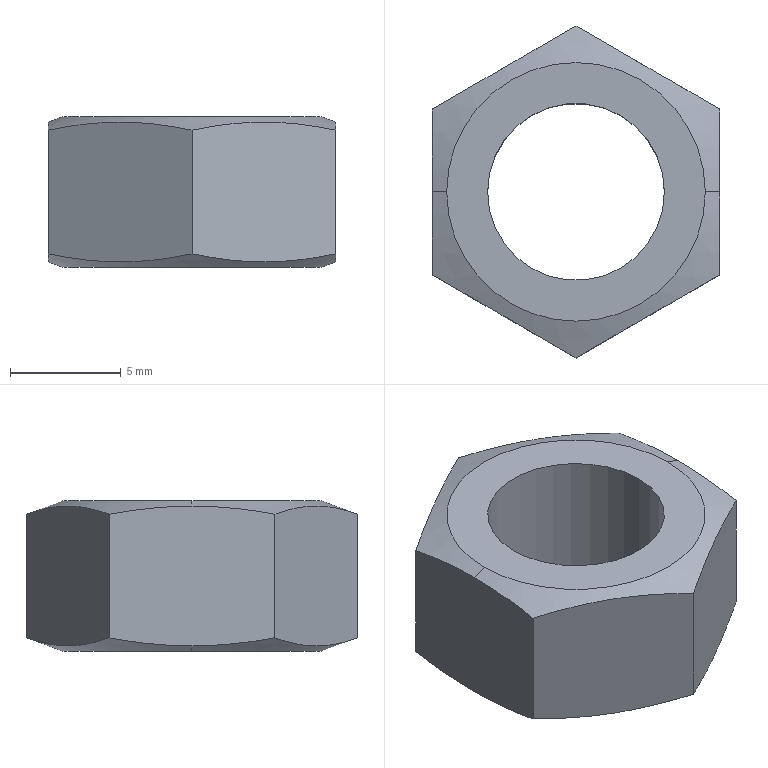Part | SolidWorks | features Extrusion 1, ICE 1, MirrorPattern 1, RefAxis 1, RevCut 1 | 1 solid | 14 faces | box 13 x 15.011 x 6.8 mm | volume 637.901 mm3 | plane 8 | cone 4 | cylinder 2 | commonest cylinder face diameters 8 x2
STEP:
#1=CARTESIAN_POINT('',(-4.,0.,0.));
#2=VERTEX_POINT('',#1);
#3=CARTESIAN_POINT('',(4.,0.,0.));
#4=VERTEX_POINT('',#3);
#5=CARTESIAN_POINT('',(0.,0.,0.));
#6=DIRECTION('',(0.,0.,1.));
#7=DIRECTION('',(1.,0.,0.));
#8=AXIS2_PLACEMENT_3D('',#5,#6,#7);
#9=CIRCLE('',#8,4.);
#10=EDGE_CURVE('',#2,#4,#9,.T.);
#11=ORIENTED_EDGE('',*,*,#10,.F.);
#12=CARTESIAN_POINT('',(-4.,0.,6.8));
#13=VERTEX_POINT('',#12);
#14=CARTESIAN_POINT('',(-4.,0.,0.));
#15=DIRECTION('',(0.,0.,1.));
#16=VECTOR('',#15,1000.);
#17=LINE('',#14,#16);
#18=EDGE_CURVE('',#2,#13,#17,.T.);
#19=ORIENTED_EDGE('',*,*,#18,.T.);
#20=CARTESIAN_POINT('',(4.,0.,6.8));
#21=VERTEX_POINT('',#20);
#22=CARTESIAN_POINT('',(0.,0.,6.8));
#23=DIRECTION('',(0.,0.,1.));
#24=DIRECTION('',(1.,0.,0.));
#25=AXIS2_PLACEMENT_3D('',#22,#23,#24);
#26=CIRCLE('',#25,4.);
#27=EDGE_CURVE('',#13,#21,#26,.T.);
#28=ORIENTED_EDGE('',*,*,#27,.T.);
#29=CARTESIAN_POINT('',(4.,0.,0.));
#30=DIRECTION('',(0.,0.,1.));
#31=VECTOR('',#30,1000.);
#32=LINE('',#29,#31);
#33=EDGE_CURVE('',#4,#21,#32,.T.);
#34=ORIENTED_EDGE('',*,*,#33,.F.);
#35=EDGE_LOOP('',(#11,#19,#28,#34));
#36=FACE_OUTER_BOUND('',#35,.T.);
#37=CARTESIAN_POINT('',(0.,0.,0.));
#38=DIRECTION('',(0.,0.,1.));
#39=DIRECTION('',(1.,0.,0.));
#40=AXIS2_PLACEMENT_3D('',#37,#38,#39);
#41=CYLINDRICAL_SURFACE('',#40,4.);
#42=ADVANCED_FACE('',(#36),#41,.F.);
#43=CARTESIAN_POINT('',(-5.85,0.,0.));
#44=VERTEX_POINT('',#43);
#45=CARTESIAN_POINT('',(5.85,0.,0.));
#46=VERTEX_POINT('',#45);
#47=CARTESIAN_POINT('',(0.,0.,0.));
#48=DIRECTION('',(0.,0.,1.));
#49=DIRECTION('',(1.,0.,0.));
#50=AXIS2_PLACEMENT_3D('',#47,#48,#49);
#51=CIRCLE('',#50,5.85);
#52=EDGE_CURVE('',#44,#46,#51,.T.);
#53=ORIENTED_EDGE('',*,*,#52,.T.);
#54=CARTESIAN_POINT('',(6.5,0.,0.2366));
#55=VERTEX_POINT('',#54);
#56=CARTESIAN_POINT('',(7.506,0.,0.6026));
#57=DIRECTION('',(0.9397,0.,0.342));
#58=VECTOR('',#57,1000.);
#59=LINE('',#56,#58);
#60=EDGE_CURVE('',#46,#55,#59,.T.);
#61=ORIENTED_EDGE('',*,*,#60,.T.);
#62=CARTESIAN_POINT('',(6.5,-3.753,0.6026));
#63=VERTEX_POINT('',#62);
#64=CARTESIAN_POINT('',(6.5,-3.753,0.6026));
#65=CARTESIAN_POINT('',(6.5,-3.131,0.4895));
#66=CARTESIAN_POINT('',(6.5,-2.503,0.3965));
#67=CARTESIAN_POINT('',(6.5,-1.251,0.27));
#68=CARTESIAN_POINT('',(6.5,-0.6249,0.2366));
#69=CARTESIAN_POINT('',(6.5,0.,0.2366));
#70=B_SPLINE_CURVE_WITH_KNOTS('',3,(#64,#65,#66,#67,#68,#69),.UNSPECIFIED.,.F.,.F.,(4,2,4),(0.00636,0.008252,0.01014),.UNSPECIFIED.);
#71=EDGE_CURVE('',#63,#55,#70,.T.);
#72=ORIENTED_EDGE('',*,*,#71,.F.);
#73=CARTESIAN_POINT('',(0.,-7.506,0.6026));
#74=VERTEX_POINT('',#73);
#75=CARTESIAN_POINT('',(0.,-7.506,0.6026));
#76=CARTESIAN_POINT('',(0.5417,-7.193,0.4887));
#77=CARTESIAN_POINT('',(1.083,-6.88,0.3963));
#78=CARTESIAN_POINT('',(2.167,-6.255,0.27));
#79=CARTESIAN_POINT('',(3.25,-5.629,0.2031));
#80=CARTESIAN_POINT('',(4.333,-5.004,0.27));
#81=CARTESIAN_POINT('',(5.417,-4.378,0.3963));
#82=CARTESIAN_POINT('',(5.958,-4.066,0.4887));
#83=CARTESIAN_POINT('',(6.5,-3.753,0.6026));
#84=B_SPLINE_CURVE_WITH_KNOTS('',3,(#75,#76,#77,#78,#79,#80,#81,#82,#83),.UNSPECIFIED.,.F.,.F.,(4,2,1,2,4),(0.000000231,0.001877,0.003753,0.005629,0.007506),.UNSPECIFIED.);
#85=EDGE_CURVE('',#74,#63,#84,.T.);
#86=ORIENTED_EDGE('',*,*,#85,.F.);
#87=CARTESIAN_POINT('',(-6.5,-3.753,0.6026));
#88=VERTEX_POINT('',#87);
#89=CARTESIAN_POINT('',(-6.5,-3.753,0.6026));
#90=CARTESIAN_POINT('',(-5.958,-4.066,0.4887));
#91=CARTESIAN_POINT('',(-5.417,-4.378,0.3963));
#92=CARTESIAN_POINT('',(-4.333,-5.004,0.27));
#93=CARTESIAN_POINT('',(-3.25,-5.629,0.2031));
#94=CARTESIAN_POINT('',(-2.167,-6.255,0.27));
#95=CARTESIAN_POINT('',(-1.083,-6.88,0.3963));
#96=CARTESIAN_POINT('',(-0.5417,-7.193,0.4887));
#97=CARTESIAN_POINT('',(0.,-7.506,0.6026));
#98=B_SPLINE_CURVE_WITH_KNOTS('',3,(#89,#90,#91,#92,#93,#94,#95,#96,#97),.UNSPECIFIED.,.F.,.F.,(4,2,1,2,4),(0.000000231,0.001877,0.003753,0.005629,0.007506),.UNSPECIFIED.);
#99=EDGE_CURVE('',#88,#74,#98,.T.);
#100=ORIENTED_EDGE('',*,*,#99,.F.);
#101=CARTESIAN_POINT('',(-6.5,0.,0.2366));
#102=VERTEX_POINT('',#101);
#103=CARTESIAN_POINT('',(-6.5,0.,0.2366));
#104=CARTESIAN_POINT('',(-6.5,-0.6249,0.2366));
#105=CARTESIAN_POINT('',(-6.5,-1.251,0.27));
#106=CARTESIAN_POINT('',(-6.5,-2.503,0.3965));
#107=CARTESIAN_POINT('',(-6.5,-3.131,0.4895));
#108=CARTESIAN_POINT('',(-6.5,-3.753,0.6026));
#109=B_SPLINE_CURVE_WITH_KNOTS('',3,(#103,#104,#105,#106,#107,#108),.UNSPECIFIED.,.F.,.F.,(4,2,4),(0.0174,0.01929,0.02117),.UNSPECIFIED.);
#110=EDGE_CURVE('',#102,#88,#109,.T.);
#111=ORIENTED_EDGE('',*,*,#110,.F.);
#112=CARTESIAN_POINT('',(-7.506,0.,0.6026));
#113=DIRECTION('',(-0.9397,0.,0.342));
#114=VECTOR('',#113,1000.);
#115=LINE('',#112,#114);
#116=EDGE_CURVE('',#44,#102,#115,.T.);
#117=ORIENTED_EDGE('',*,*,#116,.F.);
#118=EDGE_LOOP('',(#53,#61,#72,#86,#100,#111,#117));
#119=FACE_OUTER_BOUND('',#118,.T.);
#120=CARTESIAN_POINT('',(0.,0.,0.6026));
#121=DIRECTION('',(0.,0.,1.));
#122=DIRECTION('',(-1.,0.,0.));
#123=AXIS2_PLACEMENT_3D('',#120,#121,#122);
#124=CONICAL_SURFACE('',#123,7.506,1.222);
#125=ADVANCED_FACE('',(#119),#124,.T.);
#126=CARTESIAN_POINT('',(5.85,0.,6.8));
#127=VERTEX_POINT('',#126);
#128=CARTESIAN_POINT('',(-5.85,0.,6.8));
#129=VERTEX_POINT('',#128);
#130=CARTESIAN_POINT('',(0.,0.,6.8));
#131=DIRECTION('',(0.,0.,1.));
#132=DIRECTION('',(1.,0.,0.));
#133=AXIS2_PLACEMENT_3D('',#130,#131,#132);
#134=CIRCLE('',#133,5.85);
#135=EDGE_CURVE('',#127,#129,#134,.T.);
#136=ORIENTED_EDGE('',*,*,#135,.F.);
#137=CARTESIAN_POINT('',(6.5,0.,6.563));
#138=VERTEX_POINT('',#137);
#139=CARTESIAN_POINT('',(7.506,0.,6.197));
#140=DIRECTION('',(0.9397,0.,-0.342));
#141=VECTOR('',#140,1000.);
#142=LINE('',#139,#141);
#143=EDGE_CURVE('',#127,#138,#142,.T.);
#144=ORIENTED_EDGE('',*,*,#143,.T.);
#145=CARTESIAN_POINT('',(6.5,3.753,6.197));
#146=VERTEX_POINT('',#145);
#147=CARTESIAN_POINT('',(6.5,3.753,6.197));
#148=CARTESIAN_POINT('',(6.5,3.129,6.311));
#149=CARTESIAN_POINT('',(6.5,2.504,6.403));
#150=CARTESIAN_POINT('',(6.5,1.253,6.53));
#151=CARTESIAN_POINT('',(6.5,0.6268,6.563));
#152=CARTESIAN_POINT('',(6.5,0.,6.563));
#153=B_SPLINE_CURVE_WITH_KNOTS('',3,(#147,#148,#149,#150,#151,#152),.UNSPECIFIED.,.F.,.F.,(4,2,4),(0.01362,0.01551,0.0174),.UNSPECIFIED.);
#154=EDGE_CURVE('',#146,#138,#153,.T.);
#155=ORIENTED_EDGE('',*,*,#154,.F.);
#156=CARTESIAN_POINT('',(0.,7.506,6.197));
#157=VERTEX_POINT('',#156);
#158=CARTESIAN_POINT('',(0.,7.506,6.197));
#159=CARTESIAN_POINT('',(0.5417,7.193,6.311));
#160=CARTESIAN_POINT('',(1.083,6.88,6.404));
#161=CARTESIAN_POINT('',(2.167,6.255,6.53));
#162=CARTESIAN_POINT('',(3.25,5.629,6.597));
#163=CARTESIAN_POINT('',(4.333,5.004,6.53));
#164=CARTESIAN_POINT('',(5.417,4.378,6.404));
#165=CARTESIAN_POINT('',(5.958,4.066,6.311));
#166=CARTESIAN_POINT('',(6.5,3.753,6.197));
#167=B_SPLINE_CURVE_WITH_KNOTS('',3,(#158,#159,#160,#161,#162,#163,#164,#165,#166),.UNSPECIFIED.,.F.,.F.,(4,2,1,2,4),(0.000000231,0.001877,0.003753,0.005629,0.007506),.UNSPECIFIED.);
#168=EDGE_CURVE('',#157,#146,#167,.T.);
#169=ORIENTED_EDGE('',*,*,#168,.F.);
#170=CARTESIAN_POINT('',(-6.5,3.753,6.197));
#171=VERTEX_POINT('',#170);
#172=CARTESIAN_POINT('',(-6.5,3.753,6.197));
#173=CARTESIAN_POINT('',(-5.958,4.066,6.311));
#174=CARTESIAN_POINT('',(-5.417,4.378,6.404));
#175=CARTESIAN_POINT('',(-4.333,5.004,6.53));
#176=CARTESIAN_POINT('',(-3.25,5.629,6.597));
#177=CARTESIAN_POINT('',(-2.167,6.255,6.53));
#178=CARTESIAN_POINT('',(-1.083,6.88,6.404));
#179=CARTESIAN_POINT('',(-0.5417,7.193,6.311));
#180=CARTESIAN_POINT('',(0.,7.506,6.197));
#181=B_SPLINE_CURVE_WITH_KNOTS('',3,(#172,#173,#174,#175,#176,#177,#178,#179,#180),.UNSPECIFIED.,.F.,.F.,(4,2,1,2,4),(0.000000231,0.001877,0.003753,0.005629,0.007506),.UNSPECIFIED.);
#182=EDGE_CURVE('',#171,#157,#181,.T.);
#183=ORIENTED_EDGE('',*,*,#182,.F.);
#184=CARTESIAN_POINT('',(-6.5,0.,6.563));
#185=VERTEX_POINT('',#184);
#186=CARTESIAN_POINT('',(-6.5,0.,6.563));
#187=CARTESIAN_POINT('',(-6.5,0.6268,6.563));
#188=CARTESIAN_POINT('',(-6.5,1.253,6.53));
#189=CARTESIAN_POINT('',(-6.5,2.504,6.403));
#190=CARTESIAN_POINT('',(-6.5,3.129,6.311));
#191=CARTESIAN_POINT('',(-6.5,3.753,6.197));
#192=B_SPLINE_CURVE_WITH_KNOTS('',3,(#186,#187,#188,#189,#190,#191),.UNSPECIFIED.,.F.,.F.,(4,2,4),(0.01014,0.01204,0.01394),.UNSPECIFIED.);
#193=EDGE_CURVE('',#185,#171,#192,.T.);
#194=ORIENTED_EDGE('',*,*,#193,.F.);
#195=CARTESIAN_POINT('',(-7.506,0.,6.197));
#196=DIRECTION('',(-0.9397,0.,-0.342));
#197=VECTOR('',#196,1000.);
#198=LINE('',#195,#197);
#199=EDGE_CURVE('',#129,#185,#198,.T.);
#200=ORIENTED_EDGE('',*,*,#199,.F.);
#201=EDGE_LOOP('',(#136,#144,#155,#169,#183,#194,#200));
#202=FACE_OUTER_BOUND('',#201,.T.);
#203=CARTESIAN_POINT('',(0.,0.,6.197));
#204=DIRECTION('',(0.,0.,-1.));
#205=DIRECTION('',(-1.,0.,0.));
#206=AXIS2_PLACEMENT_3D('',#203,#204,#205);
#207=CONICAL_SURFACE('',#206,7.506,1.222);
#208=ADVANCED_FACE('',(#202),#207,.T.);
#209=CARTESIAN_POINT('',(6.5,3.753,0.6026));
#210=VERTEX_POINT('',#209);
#211=CARTESIAN_POINT('',(6.5,3.753,6.8));
#212=DIRECTION('',(0.,0.,-1.));
#213=VECTOR('',#212,1000.);
#214=LINE('',#211,#213);
#215=EDGE_CURVE('',#146,#210,#214,.T.);
#216=ORIENTED_EDGE('',*,*,#215,.T.);
#217=CARTESIAN_POINT('',(0.,7.506,0.6026));
#218=VERTEX_POINT('',#217);
#219=CARTESIAN_POINT('',(6.5,3.753,0.6026));
#220=CARTESIAN_POINT('',(5.958,4.066,0.4887));
#221=CARTESIAN_POINT('',(5.417,4.378,0.3963));
#222=CARTESIAN_POINT('',(4.333,5.004,0.27));
#223=CARTESIAN_POINT('',(3.25,5.629,0.2031));
#224=CARTESIAN_POINT('',(2.167,6.255,0.27));
#225=CARTESIAN_POINT('',(1.083,6.88,0.3963));
#226=CARTESIAN_POINT('',(0.5417,7.193,0.4887));
#227=CARTESIAN_POINT('',(0.,7.506,0.6026));
#228=B_SPLINE_CURVE_WITH_KNOTS('',3,(#219,#220,#221,#222,#223,#224,#225,#226,#227),.UNSPECIFIED.,.F.,.F.,(4,2,1,2,4),(0.000000231,0.001877,0.003753,0.005629,0.007506),.UNSPECIFIED.);
#229=EDGE_CURVE('',#210,#218,#228,.T.);
#230=ORIENTED_EDGE('',*,*,#229,.T.);
#231=CARTESIAN_POINT('',(0.,7.506,6.8));
#232=DIRECTION('',(0.,0.,-1.));
#233=VECTOR('',#232,1000.);
#234=LINE('',#231,#233);
#235=EDGE_CURVE('',#157,#218,#234,.T.);
#236=ORIENTED_EDGE('',*,*,#235,.F.);
#237=ORIENTED_EDGE('',*,*,#168,.T.);
#238=EDGE_LOOP('',(#216,#230,#236,#237));
#239=FACE_OUTER_BOUND('',#238,.T.);
#240=CARTESIAN_POINT('',(6.5,3.753,6.8));
#241=DIRECTION('',(-0.5,-0.866,0.));
#242=DIRECTION('',(0.866,-0.5,0.));
#243=AXIS2_PLACEMENT_3D('',#240,#241,#242);
#244=PLANE('',#243);
#245=ADVANCED_FACE('',(#239),#244,.F.);
#246=ORIENTED_EDGE('',*,*,#235,.T.);
#247=CARTESIAN_POINT('',(-6.5,3.753,0.6026));
#248=VERTEX_POINT('',#247);
#249=CARTESIAN_POINT('',(0.,7.506,0.6026));
#250=CARTESIAN_POINT('',(-0.5417,7.193,0.4887));
#251=CARTESIAN_POINT('',(-1.083,6.88,0.3963));
#252=CARTESIAN_POINT('',(-2.167,6.255,0.27));
#253=CARTESIAN_POINT('',(-3.25,5.629,0.2031));
#254=CARTESIAN_POINT('',(-4.333,5.004,0.27));
#255=CARTESIAN_POINT('',(-5.417,4.378,0.3963));
#256=CARTESIAN_POINT('',(-5.958,4.066,0.4887));
#257=CARTESIAN_POINT('',(-6.5,3.753,0.6026));
#258=B_SPLINE_CURVE_WITH_KNOTS('',3,(#249,#250,#251,#252,#253,#254,#255,#256,#257),.UNSPECIFIED.,.F.,.F.,(4,2,1,2,4),(0.000000231,0.001877,0.003753,0.005629,0.007506),.UNSPECIFIED.);
#259=EDGE_CURVE('',#218,#248,#258,.T.);
#260=ORIENTED_EDGE('',*,*,#259,.T.);
#261=CARTESIAN_POINT('',(-6.5,3.753,6.8));
#262=DIRECTION('',(0.,0.,-1.));
#263=VECTOR('',#262,1000.);
#264=LINE('',#261,#263);
#265=EDGE_CURVE('',#171,#248,#264,.T.);
#266=ORIENTED_EDGE('',*,*,#265,.F.);
#267=ORIENTED_EDGE('',*,*,#182,.T.);
#268=EDGE_LOOP('',(#246,#260,#266,#267));
#269=FACE_OUTER_BOUND('',#268,.T.);
#270=CARTESIAN_POINT('',(0.,7.506,6.8));
#271=DIRECTION('',(0.5,-0.866,0.));
#272=DIRECTION('',(0.866,0.5,0.));
#273=AXIS2_PLACEMENT_3D('',#270,#271,#272);
#274=PLANE('',#273);
#275=ADVANCED_FACE('',(#269),#274,.F.);
#276=ORIENTED_EDGE('',*,*,#265,.T.);
#277=CARTESIAN_POINT('',(-6.5,3.753,0.6026));
#278=CARTESIAN_POINT('',(-6.5,3.129,0.4891));
#279=CARTESIAN_POINT('',(-6.5,2.504,0.3966));
#280=CARTESIAN_POINT('',(-6.5,1.253,0.2702));
#281=CARTESIAN_POINT('',(-6.5,0.6268,0.2366));
#282=CARTESIAN_POINT('',(-6.5,0.,0.2366));
#283=B_SPLINE_CURVE_WITH_KNOTS('',3,(#277,#278,#279,#280,#281,#282),.UNSPECIFIED.,.F.,.F.,(4,2,4),(0.01362,0.01551,0.0174),.UNSPECIFIED.);
#284=EDGE_CURVE('',#248,#102,#283,.T.);
#285=ORIENTED_EDGE('',*,*,#284,.T.);
#286=ORIENTED_EDGE('',*,*,#110,.T.);
#287=CARTESIAN_POINT('',(-6.5,-3.753,6.197));
#288=VERTEX_POINT('',#287);
#289=CARTESIAN_POINT('',(-6.5,-3.753,6.8));
#290=DIRECTION('',(0.,0.,-1.));
#291=VECTOR('',#290,1000.);
#292=LINE('',#289,#291);
#293=EDGE_CURVE('',#288,#88,#292,.T.);
#294=ORIENTED_EDGE('',*,*,#293,.F.);
#295=CARTESIAN_POINT('',(-6.5,-3.753,6.197));
#296=CARTESIAN_POINT('',(-6.5,-3.131,6.31));
#297=CARTESIAN_POINT('',(-6.5,-2.503,6.404));
#298=CARTESIAN_POINT('',(-6.5,-1.251,6.53));
#299=CARTESIAN_POINT('',(-6.5,-0.6249,6.563));
#300=CARTESIAN_POINT('',(-6.5,0.,6.563));
#301=B_SPLINE_CURVE_WITH_KNOTS('',3,(#295,#296,#297,#298,#299,#300),.UNSPECIFIED.,.F.,.F.,(4,2,4),(0.00636,0.008252,0.01014),.UNSPECIFIED.);
#302=EDGE_CURVE('',#288,#185,#301,.T.);
#303=ORIENTED_EDGE('',*,*,#302,.T.);
#304=ORIENTED_EDGE('',*,*,#193,.T.);
#305=EDGE_LOOP('',(#276,#285,#286,#294,#303,#304));
#306=FACE_OUTER_BOUND('',#305,.T.);
#307=CARTESIAN_POINT('',(-6.5,3.753,6.8));
#308=DIRECTION('',(1.,0.,0.));
#309=DIRECTION('',(0.,0.,-1.));
#310=AXIS2_PLACEMENT_3D('',#307,#308,#309);
#311=PLANE('',#310);
#312=ADVANCED_FACE('',(#306),#311,.F.);
#313=ORIENTED_EDGE('',*,*,#293,.T.);
#314=ORIENTED_EDGE('',*,*,#99,.T.);
#315=CARTESIAN_POINT('',(0.,-7.506,6.197));
#316=VERTEX_POINT('',#315);
#317=CARTESIAN_POINT('',(0.,-7.506,6.8));
#318=DIRECTION('',(0.,0.,-1.));
#319=VECTOR('',#318,1000.);
#320=LINE('',#317,#319);
#321=EDGE_CURVE('',#316,#74,#320,.T.);
#322=ORIENTED_EDGE('',*,*,#321,.F.);
#323=CARTESIAN_POINT('',(0.,-7.506,6.197));
#324=CARTESIAN_POINT('',(-0.5417,-7.193,6.311));
#325=CARTESIAN_POINT('',(-1.083,-6.88,6.404));
#326=CARTESIAN_POINT('',(-2.167,-6.255,6.53));
#327=CARTESIAN_POINT('',(-3.25,-5.629,6.597));
#328=CARTESIAN_POINT('',(-4.333,-5.004,6.53));
#329=CARTESIAN_POINT('',(-5.417,-4.378,6.404));
#330=CARTESIAN_POINT('',(-5.958,-4.066,6.311));
#331=CARTESIAN_POINT('',(-6.5,-3.753,6.197));
#332=B_SPLINE_CURVE_WITH_KNOTS('',3,(#323,#324,#325,#326,#327,#328,#329,#330,#331),.UNSPECIFIED.,.F.,.F.,(4,2,1,2,4),(0.000000231,0.001877,0.003753,0.005629,0.007506),.UNSPECIFIED.);
#333=EDGE_CURVE('',#316,#288,#332,.T.);
#334=ORIENTED_EDGE('',*,*,#333,.T.);
#335=EDGE_LOOP('',(#313,#314,#322,#334));
#336=FACE_OUTER_BOUND('',#335,.T.);
#337=CARTESIAN_POINT('',(-6.5,-3.753,6.8));
#338=DIRECTION('',(0.5,0.866,0.));
#339=DIRECTION('',(-0.866,0.5,0.));
#340=AXIS2_PLACEMENT_3D('',#337,#338,#339);
#341=PLANE('',#340);
#342=ADVANCED_FACE('',(#336),#341,.F.);
#343=ORIENTED_EDGE('',*,*,#321,.T.);
#344=ORIENTED_EDGE('',*,*,#85,.T.);
#345=CARTESIAN_POINT('',(6.5,-3.753,6.197));
#346=VERTEX_POINT('',#345);
#347=CARTESIAN_POINT('',(6.5,-3.753,6.8));
#348=DIRECTION('',(0.,0.,-1.));
#349=VECTOR('',#348,1000.);
#350=LINE('',#347,#349);
#351=EDGE_CURVE('',#346,#63,#350,.T.);
#352=ORIENTED_EDGE('',*,*,#351,.F.);
#353=CARTESIAN_POINT('',(6.5,-3.753,6.197));
#354=CARTESIAN_POINT('',(5.958,-4.066,6.311));
#355=CARTESIAN_POINT('',(5.417,-4.378,6.404));
#356=CARTESIAN_POINT('',(4.333,-5.004,6.53));
#357=CARTESIAN_POINT('',(3.25,-5.629,6.597));
#358=CARTESIAN_POINT('',(2.167,-6.255,6.53));
#359=CARTESIAN_POINT('',(1.083,-6.88,6.404));
#360=CARTESIAN_POINT('',(0.5417,-7.193,6.311));
#361=CARTESIAN_POINT('',(0.,-7.506,6.197));
#362=B_SPLINE_CURVE_WITH_KNOTS('',3,(#353,#354,#355,#356,#357,#358,#359,#360,#361),.UNSPECIFIED.,.F.,.F.,(4,2,1,2,4),(0.000000231,0.001877,0.003753,0.005629,0.007506),.UNSPECIFIED.);
#363=EDGE_CURVE('',#346,#316,#362,.T.);
#364=ORIENTED_EDGE('',*,*,#363,.T.);
#365=EDGE_LOOP('',(#343,#344,#352,#364));
#366=FACE_OUTER_BOUND('',#365,.T.);
#367=CARTESIAN_POINT('',(0.,-7.506,6.8));
#368=DIRECTION('',(-0.5,0.866,0.));
#369=DIRECTION('',(-0.866,-0.5,0.));
#370=AXIS2_PLACEMENT_3D('',#367,#368,#369);
#371=PLANE('',#370);
#372=ADVANCED_FACE('',(#366),#371,.F.);
#373=ORIENTED_EDGE('',*,*,#351,.T.);
#374=ORIENTED_EDGE('',*,*,#71,.T.);
#375=CARTESIAN_POINT('',(6.5,0.,0.2366));
#376=CARTESIAN_POINT('',(6.5,0.6268,0.2366));
#377=CARTESIAN_POINT('',(6.5,1.253,0.2702));
#378=CARTESIAN_POINT('',(6.5,2.504,0.3966));
#379=CARTESIAN_POINT('',(6.5,3.129,0.4891));
#380=CARTESIAN_POINT('',(6.5,3.753,0.6026));
#381=B_SPLINE_CURVE_WITH_KNOTS('',3,(#375,#376,#377,#378,#379,#380),.UNSPECIFIED.,.F.,.F.,(4,2,4),(0.01014,0.01204,0.01394),.UNSPECIFIED.);
#382=EDGE_CURVE('',#55,#210,#381,.T.);
#383=ORIENTED_EDGE('',*,*,#382,.T.);
#384=ORIENTED_EDGE('',*,*,#215,.F.);
#385=ORIENTED_EDGE('',*,*,#154,.T.);
#386=CARTESIAN_POINT('',(6.5,0.,6.563));
#387=CARTESIAN_POINT('',(6.5,-0.6249,6.563));
#388=CARTESIAN_POINT('',(6.5,-1.251,6.53));
#389=CARTESIAN_POINT('',(6.5,-2.503,6.404));
#390=CARTESIAN_POINT('',(6.5,-3.131,6.31));
#391=CARTESIAN_POINT('',(6.5,-3.753,6.197));
#392=B_SPLINE_CURVE_WITH_KNOTS('',3,(#386,#387,#388,#389,#390,#391),.UNSPECIFIED.,.F.,.F.,(4,2,4),(0.0174,0.01929,0.02117),.UNSPECIFIED.);
#393=EDGE_CURVE('',#138,#346,#392,.T.);
#394=ORIENTED_EDGE('',*,*,#393,.T.);
#395=EDGE_LOOP('',(#373,#374,#383,#384,#385,#394));
#396=FACE_OUTER_BOUND('',#395,.T.);
#397=CARTESIAN_POINT('',(6.5,-3.753,6.8));
#398=DIRECTION('',(-1.,0.,0.));
#399=DIRECTION('',(0.,0.,1.));
#400=AXIS2_PLACEMENT_3D('',#397,#398,#399);
#401=PLANE('',#400);
#402=ADVANCED_FACE('',(#396),#401,.F.);
#403=ORIENTED_EDGE('',*,*,#143,.F.);
#404=CARTESIAN_POINT('',(0.,0.,6.8));
#405=DIRECTION('',(0.,0.,1.));
#406=DIRECTION('',(1.,0.,0.));
#407=AXIS2_PLACEMENT_3D('',#404,#405,#406);
#408=CIRCLE('',#407,5.85);
#409=EDGE_CURVE('',#129,#127,#408,.T.);
#410=ORIENTED_EDGE('',*,*,#409,.F.);
#411=ORIENTED_EDGE('',*,*,#199,.T.);
#412=ORIENTED_EDGE('',*,*,#302,.F.);
#413=ORIENTED_EDGE('',*,*,#333,.F.);
#414=ORIENTED_EDGE('',*,*,#363,.F.);
#415=ORIENTED_EDGE('',*,*,#393,.F.);
#416=EDGE_LOOP('',(#403,#410,#411,#412,#413,#414,#415));
#417=FACE_OUTER_BOUND('',#416,.T.);
#418=CARTESIAN_POINT('',(0.,0.,6.197));
#419=DIRECTION('',(0.,0.,-1.));
#420=DIRECTION('',(-1.,0.,0.));
#421=AXIS2_PLACEMENT_3D('',#418,#419,#420);
#422=CONICAL_SURFACE('',#421,7.506,1.222);
#423=ADVANCED_FACE('',(#417),#422,.T.);
#424=CARTESIAN_POINT('',(0.,0.,6.8));
#425=DIRECTION('',(0.,0.,1.));
#426=DIRECTION('',(1.,0.,0.));
#427=AXIS2_PLACEMENT_3D('',#424,#425,#426);
#428=CIRCLE('',#427,4.);
#429=EDGE_CURVE('',#21,#13,#428,.T.);
#430=ORIENTED_EDGE('',*,*,#429,.F.);
#431=ORIENTED_EDGE('',*,*,#27,.F.);
#432=EDGE_LOOP('',(#430,#431));
#433=FACE_BOUND('',#432,.T.);
#434=ORIENTED_EDGE('',*,*,#409,.T.);
#435=ORIENTED_EDGE('',*,*,#135,.T.);
#436=EDGE_LOOP('',(#434,#435));
#437=FACE_OUTER_BOUND('',#436,.T.);
#438=CARTESIAN_POINT('',(0.,0.,6.8));
#439=DIRECTION('',(0.,0.,1.));
#440=DIRECTION('',(1.,0.,0.));
#441=AXIS2_PLACEMENT_3D('',#438,#439,#440);
#442=PLANE('',#441);
#443=ADVANCED_FACE('',(#433,#437),#442,.T.);
#444=ORIENTED_EDGE('',*,*,#60,.F.);
#445=CARTESIAN_POINT('',(0.,0.,0.));
#446=DIRECTION('',(0.,0.,1.));
#447=DIRECTION('',(1.,0.,0.));
#448=AXIS2_PLACEMENT_3D('',#445,#446,#447);
#449=CIRCLE('',#448,5.85);
#450=EDGE_CURVE('',#46,#44,#449,.T.);
#451=ORIENTED_EDGE('',*,*,#450,.T.);
#452=ORIENTED_EDGE('',*,*,#116,.T.);
#453=ORIENTED_EDGE('',*,*,#284,.F.);
#454=ORIENTED_EDGE('',*,*,#259,.F.);
#455=ORIENTED_EDGE('',*,*,#229,.F.);
#456=ORIENTED_EDGE('',*,*,#382,.F.);
#457=EDGE_LOOP('',(#444,#451,#452,#453,#454,#455,#456));
#458=FACE_OUTER_BOUND('',#457,.T.);
#459=CARTESIAN_POINT('',(0.,0.,0.6026));
#460=DIRECTION('',(0.,0.,1.));
#461=DIRECTION('',(-1.,0.,0.));
#462=AXIS2_PLACEMENT_3D('',#459,#460,#461);
#463=CONICAL_SURFACE('',#462,7.506,1.222);
#464=ADVANCED_FACE('',(#458),#463,.T.);
#465=CARTESIAN_POINT('',(0.,0.,0.));
#466=DIRECTION('',(0.,0.,1.));
#467=DIRECTION('',(1.,0.,0.));
#468=AXIS2_PLACEMENT_3D('',#465,#466,#467);
#469=CIRCLE('',#468,4.);
#470=EDGE_CURVE('',#4,#2,#469,.T.);
#471=ORIENTED_EDGE('',*,*,#470,.T.);
#472=ORIENTED_EDGE('',*,*,#10,.T.);
#473=EDGE_LOOP('',(#471,#472));
#474=FACE_BOUND('',#473,.T.);
#475=ORIENTED_EDGE('',*,*,#52,.F.);
#476=ORIENTED_EDGE('',*,*,#450,.F.);
#477=EDGE_LOOP('',(#475,#476));
#478=FACE_OUTER_BOUND('',#477,.T.);
#479=CARTESIAN_POINT('',(0.,0.,0.));
#480=DIRECTION('',(0.,0.,1.));
#481=DIRECTION('',(1.,0.,0.));
#482=AXIS2_PLACEMENT_3D('',#479,#480,#481);
#483=PLANE('',#482);
#484=ADVANCED_FACE('',(#474,#478),#483,.F.);
#485=ORIENTED_EDGE('',*,*,#18,.F.);
#486=ORIENTED_EDGE('',*,*,#470,.F.);
#487=ORIENTED_EDGE('',*,*,#33,.T.);
#488=ORIENTED_EDGE('',*,*,#429,.T.);
#489=EDGE_LOOP('',(#485,#486,#487,#488));
#490=FACE_OUTER_BOUND('',#489,.T.);
#491=CARTESIAN_POINT('',(0.,0.,0.));
#492=DIRECTION('',(0.,0.,1.));
#493=DIRECTION('',(1.,0.,0.));
#494=AXIS2_PLACEMENT_3D('',#491,#492,#493);
#495=CYLINDRICAL_SURFACE('',#494,4.);
#496=ADVANCED_FACE('',(#490),#495,.F.);
#497=CLOSED_SHELL('',(#42,#125,#208,#245,#275,#312,#342,#372,#402,#423,#443,#464,#484,#496));
#498=MANIFOLD_SOLID_BREP('',#497);
#499=CARTESIAN_POINT('',(0.,0.,0.));
#500=DIRECTION('',(0.,0.,1.));
#501=DIRECTION('',(1.,0.,0.));
#502=AXIS2_PLACEMENT_3D('',#499,#500,#501);
#503=(LENGTH_UNIT()NAMED_UNIT(*)SI_UNIT(.MILLI.,.METRE.));
#504=UNCERTAINTY_MEASURE_WITH_UNIT(LENGTH_MEASURE(0.00001),#503,'','');
#505=(NAMED_UNIT(*)PLANE_ANGLE_UNIT()SI_UNIT($,.RADIAN.));
#506=(NAMED_UNIT(*)SI_UNIT($,.STERADIAN.)SOLID_ANGLE_UNIT());
#507=(GEOMETRIC_REPRESENTATION_CONTEXT(3)GLOBAL_UNCERTAINTY_ASSIGNED_CONTEXT((#504))GLOBAL_UNIT_ASSIGNED_CONTEXT((#503,#505,#506))REPRESENTATION_CONTEXT('',''));
#508=ADVANCED_BREP_SHAPE_REPRESENTATION('',(#498,#502),#507);